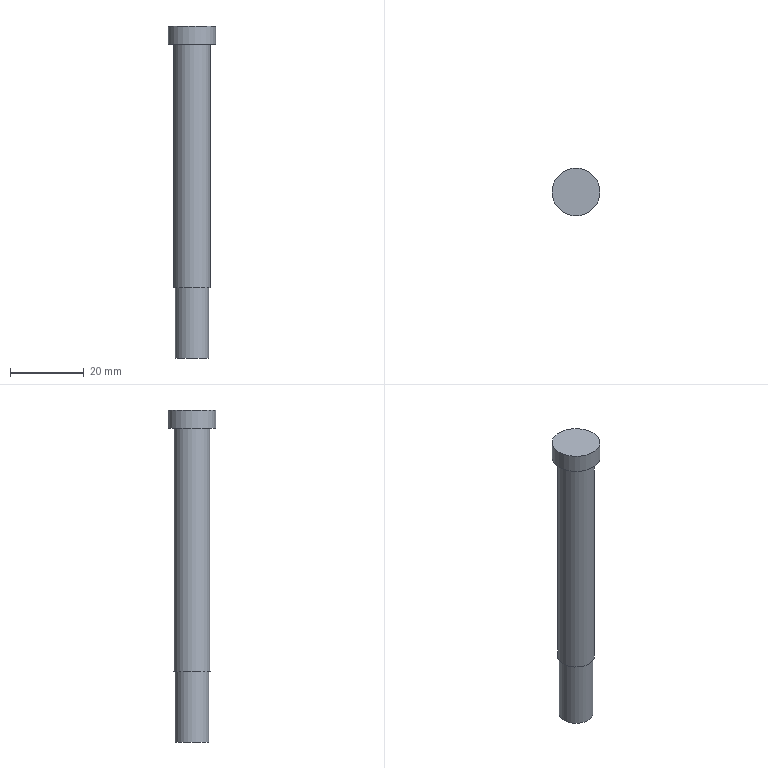Part | NX | features solid 2 | 1 solid | 7 faces | box 13 x 13 x 90 mm | volume 7083 mm3 | plane 4 | cylinder 3 | commonest cylinder face diameters 9.1 x1 10 x1 13 x1
STEP:
#1=CARTESIAN_POINT('',(-152.412,669.726,29.));
#2=VERTEX_POINT('',#1);
#3=CARTESIAN_POINT('',(-157.412,669.726,29.));
#4=DIRECTION('',(0.,0.,1.));
#5=DIRECTION('',(1.,0.,0.));
#6=AXIS2_PLACEMENT_3D('',#3,#4,#5);
#7=CIRCLE('',#6,5.);
#8=EDGE_CURVE('',#2,#2,#7,.T.);
#9=ORIENTED_EDGE('',*,*,#8,.T.);
#10=EDGE_LOOP('',(#9));
#11=FACE_BOUND('',#10,.T.);
#12=CARTESIAN_POINT('',(-152.412,669.726,95.));
#13=VERTEX_POINT('',#12);
#14=CARTESIAN_POINT('',(-157.412,669.726,95.));
#15=DIRECTION('',(0.,0.,1.));
#16=DIRECTION('',(1.,0.,0.));
#17=AXIS2_PLACEMENT_3D('',#14,#15,#16);
#18=CIRCLE('',#17,5.);
#19=EDGE_CURVE('',#13,#13,#18,.T.);
#20=ORIENTED_EDGE('',*,*,#19,.F.);
#21=EDGE_LOOP('',(#20));
#22=FACE_BOUND('',#21,.T.);
#23=CARTESIAN_POINT('',(-157.412,669.726,100.));
#24=DIRECTION('',(0.,0.,-1.));
#25=DIRECTION('',(-1.,0.,0.));
#26=AXIS2_PLACEMENT_3D('',#23,#24,#25);
#27=CYLINDRICAL_SURFACE('',#26,5.);
#28=ADVANCED_FACE('',(#11,#22),#27,.T.);
#29=CARTESIAN_POINT('',(-152.862,669.726,29.));
#30=VERTEX_POINT('',#29);
#31=CARTESIAN_POINT('',(-157.412,669.726,29.));
#32=DIRECTION('',(0.,0.,1.));
#33=DIRECTION('',(1.,0.,0.));
#34=AXIS2_PLACEMENT_3D('',#31,#32,#33);
#35=CIRCLE('',#34,4.55);
#36=EDGE_CURVE('',#30,#30,#35,.T.);
#37=ORIENTED_EDGE('',*,*,#36,.T.);
#38=EDGE_LOOP('',(#37));
#39=FACE_BOUND('',#38,.T.);
#40=ORIENTED_EDGE('',*,*,#8,.F.);
#41=EDGE_LOOP('',(#40));
#42=FACE_BOUND('',#41,.T.);
#43=CARTESIAN_POINT('',(-157.412,669.726,29.));
#44=DIRECTION('',(0.,0.,1.));
#45=DIRECTION('',(1.,0.,0.));
#46=AXIS2_PLACEMENT_3D('',#43,#44,#45);
#47=PLANE('',#46);
#48=ADVANCED_FACE('',(#39,#42),#47,.F.);
#49=CARTESIAN_POINT('',(-150.912,669.726,95.));
#50=VERTEX_POINT('',#49);
#51=CARTESIAN_POINT('',(-157.412,669.726,95.));
#52=DIRECTION('',(0.,0.,1.));
#53=DIRECTION('',(1.,0.,0.));
#54=AXIS2_PLACEMENT_3D('',#51,#52,#53);
#55=CIRCLE('',#54,6.5);
#56=EDGE_CURVE('',#50,#50,#55,.T.);
#57=ORIENTED_EDGE('',*,*,#56,.F.);
#58=EDGE_LOOP('',(#57));
#59=FACE_BOUND('',#58,.T.);
#60=ORIENTED_EDGE('',*,*,#19,.T.);
#61=EDGE_LOOP('',(#60));
#62=FACE_BOUND('',#61,.T.);
#63=CARTESIAN_POINT('',(-157.412,669.726,95.));
#64=DIRECTION('',(0.,0.,1.));
#65=DIRECTION('',(1.,0.,0.));
#66=AXIS2_PLACEMENT_3D('',#63,#64,#65);
#67=PLANE('',#66);
#68=ADVANCED_FACE('',(#59,#62),#67,.F.);
#69=ORIENTED_EDGE('',*,*,#56,.T.);
#70=EDGE_LOOP('',(#69));
#71=FACE_BOUND('',#70,.T.);
#72=CARTESIAN_POINT('',(-150.912,669.726,100.));
#73=VERTEX_POINT('',#72);
#74=CARTESIAN_POINT('',(-157.412,669.726,100.));
#75=DIRECTION('',(0.,0.,1.));
#76=DIRECTION('',(1.,0.,0.));
#77=AXIS2_PLACEMENT_3D('',#74,#75,#76);
#78=CIRCLE('',#77,6.5);
#79=EDGE_CURVE('',#73,#73,#78,.T.);
#80=ORIENTED_EDGE('',*,*,#79,.F.);
#81=EDGE_LOOP('',(#80));
#82=FACE_BOUND('',#81,.T.);
#83=CARTESIAN_POINT('',(-157.412,669.726,95.));
#84=DIRECTION('',(0.,0.,1.));
#85=DIRECTION('',(1.,0.,0.));
#86=AXIS2_PLACEMENT_3D('',#83,#84,#85);
#87=CYLINDRICAL_SURFACE('',#86,6.5);
#88=ADVANCED_FACE('',(#71,#82),#87,.T.);
#89=ORIENTED_EDGE('',*,*,#79,.T.);
#90=EDGE_LOOP('',(#89));
#91=FACE_BOUND('',#90,.T.);
#92=CARTESIAN_POINT('',(-157.412,669.726,100.));
#93=DIRECTION('',(0.,0.,1.));
#94=DIRECTION('',(1.,0.,0.));
#95=AXIS2_PLACEMENT_3D('',#92,#93,#94);
#96=PLANE('',#95);
#97=ADVANCED_FACE('',(#91),#96,.T.);
#98=CARTESIAN_POINT('',(-152.862,669.726,10.));
#99=VERTEX_POINT('',#98);
#100=CARTESIAN_POINT('',(-157.412,669.726,10.));
#101=DIRECTION('',(0.,0.,1.));
#102=DIRECTION('',(1.,0.,0.));
#103=AXIS2_PLACEMENT_3D('',#100,#101,#102);
#104=CIRCLE('',#103,4.55);
#105=EDGE_CURVE('',#99,#99,#104,.T.);
#106=ORIENTED_EDGE('',*,*,#105,.T.);
#107=EDGE_LOOP('',(#106));
#108=FACE_BOUND('',#107,.T.);
#109=ORIENTED_EDGE('',*,*,#36,.F.);
#110=EDGE_LOOP('',(#109));
#111=FACE_BOUND('',#110,.T.);
#112=CARTESIAN_POINT('',(-157.412,669.726,10.));
#113=DIRECTION('',(0.,0.,1.));
#114=DIRECTION('',(1.,0.,0.));
#115=AXIS2_PLACEMENT_3D('',#112,#113,#114);
#116=CYLINDRICAL_SURFACE('',#115,4.55);
#117=ADVANCED_FACE('',(#108,#111),#116,.T.);
#118=ORIENTED_EDGE('',*,*,#105,.F.);
#119=EDGE_LOOP('',(#118));
#120=FACE_BOUND('',#119,.T.);
#121=CARTESIAN_POINT('',(-157.412,669.726,10.));
#122=DIRECTION('',(0.,0.,1.));
#123=DIRECTION('',(1.,0.,0.));
#124=AXIS2_PLACEMENT_3D('',#121,#122,#123);
#125=PLANE('',#124);
#126=ADVANCED_FACE('',(#120),#125,.F.);
#127=CLOSED_SHELL('',(#28,#48,#68,#88,#97,#117,#126));
#128=MANIFOLD_SOLID_BREP('',#127);
#129=(LENGTH_UNIT()NAMED_UNIT(*)SI_UNIT(.MILLI.,.METRE.));
#130=UNCERTAINTY_MEASURE_WITH_UNIT(LENGTH_MEASURE(0.00001),#129,'','');
#131=(NAMED_UNIT(*)PLANE_ANGLE_UNIT()SI_UNIT($,.RADIAN.));
#132=(NAMED_UNIT(*)SI_UNIT($,.STERADIAN.)SOLID_ANGLE_UNIT());
#133=(GEOMETRIC_REPRESENTATION_CONTEXT(3)GLOBAL_UNCERTAINTY_ASSIGNED_CONTEXT((#130))GLOBAL_UNIT_ASSIGNED_CONTEXT((#129,#131,#132))REPRESENTATION_CONTEXT('',''));
#134=ADVANCED_BREP_SHAPE_REPRESENTATION('',(#128),#133);